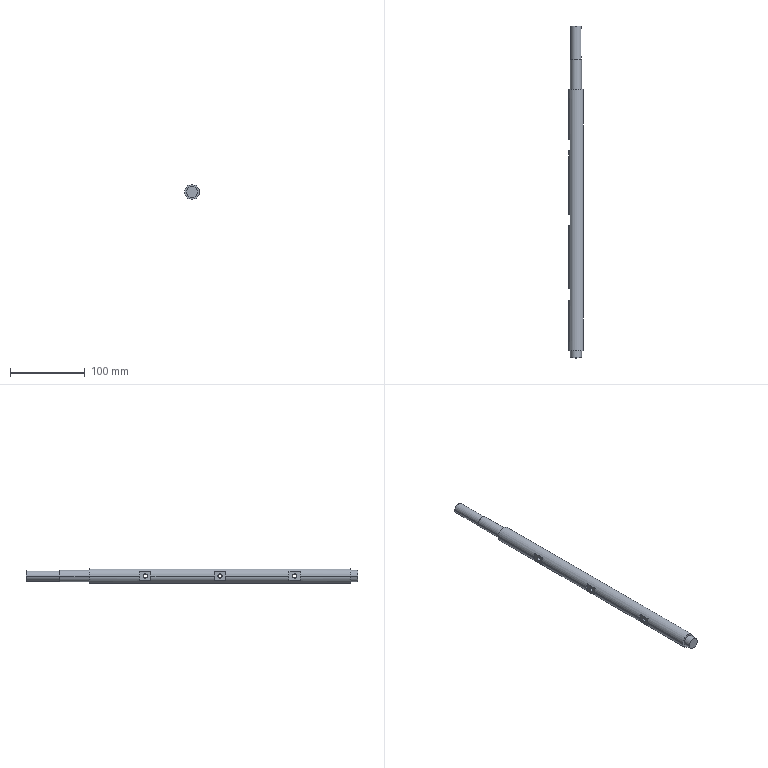Part | STEP file | B1-012 | 1 solid | 40 faces | box 20 x 445 x 20 mm | volume 123230 mm3 | cylinder 17 | plane 17 | cone 6 | commonest cylinder face diameters 5.5 x6 15 x4 5 x3 14 x2 20 x2